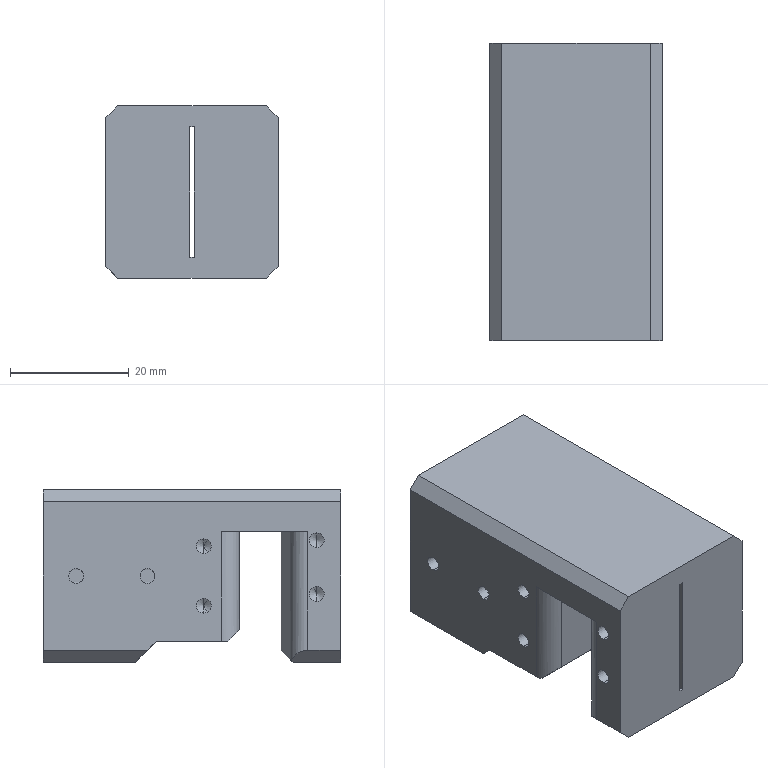Part | SolidWorks | features HoleWzd 5, ICE 5, Chamfer 4, Fillet 2, Extrusion 1 | 1 solid | 79 faces | box 29 x 50 x 29 mm | volume 27875 mm3 | plane 33 | cylinder 30 | cone 16 | commonest cylinder face diameters 2.5 x24 6 x4 16 x2